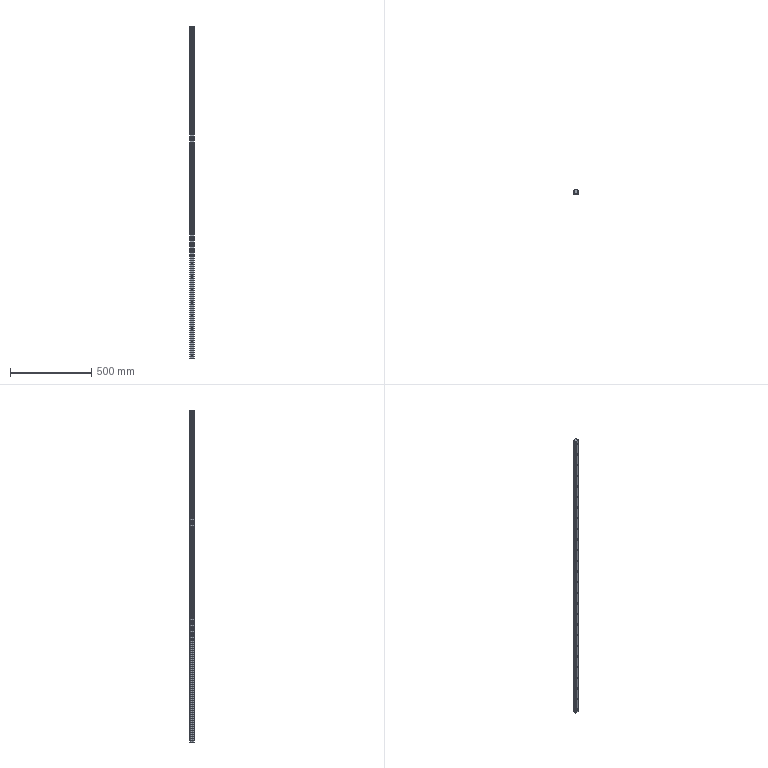Part | SolidWorks | features BaseBody 1, HoleWzd 1, ICE 1 | 1 solid | 182 faces | box 28 x 26 x 2040 mm | volume 1186082 mm3 | cylinder 126 | plane 56 | commonest cylinder face diameters 9 x52 14 x52 1.2 x12 1.6 x6 5.66 x4